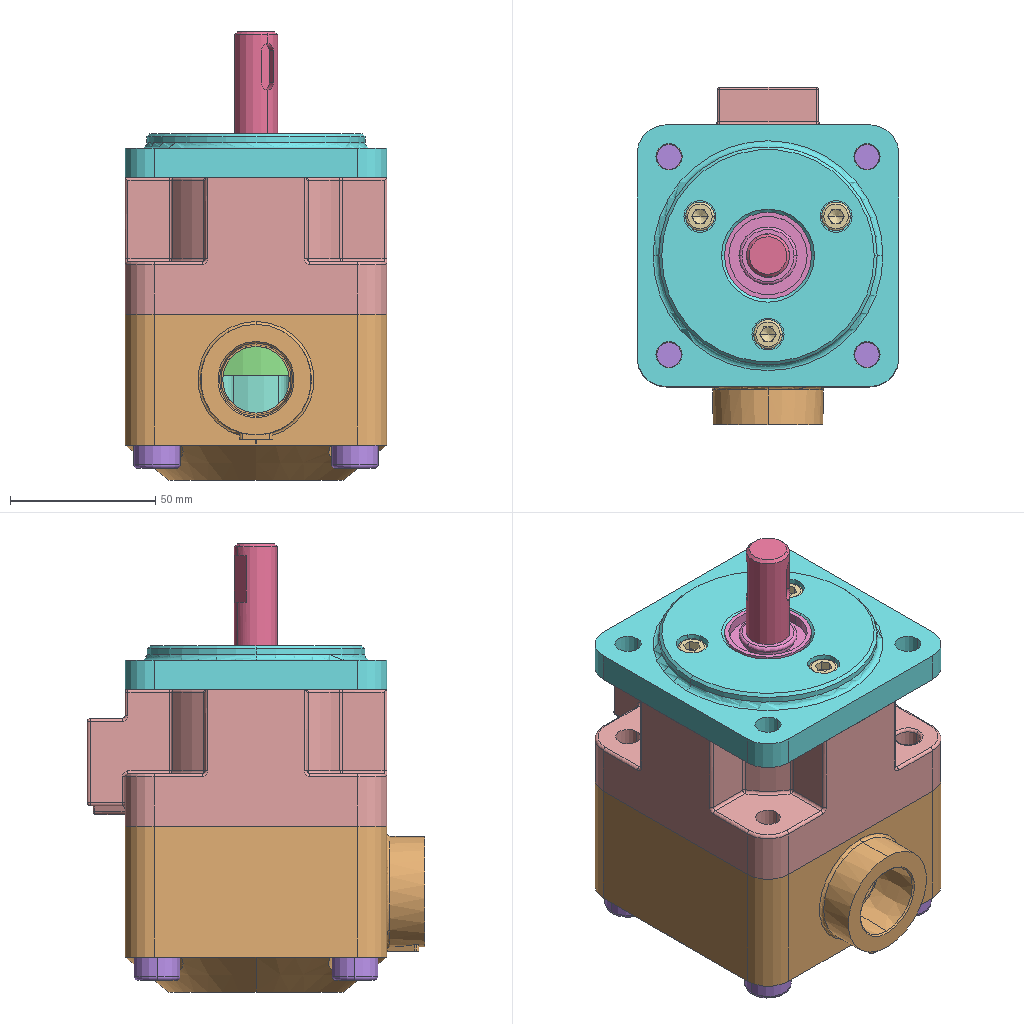Assembly | SolidWorks | 24 different items | 38 placed | box 90 x 116 x 154 mm
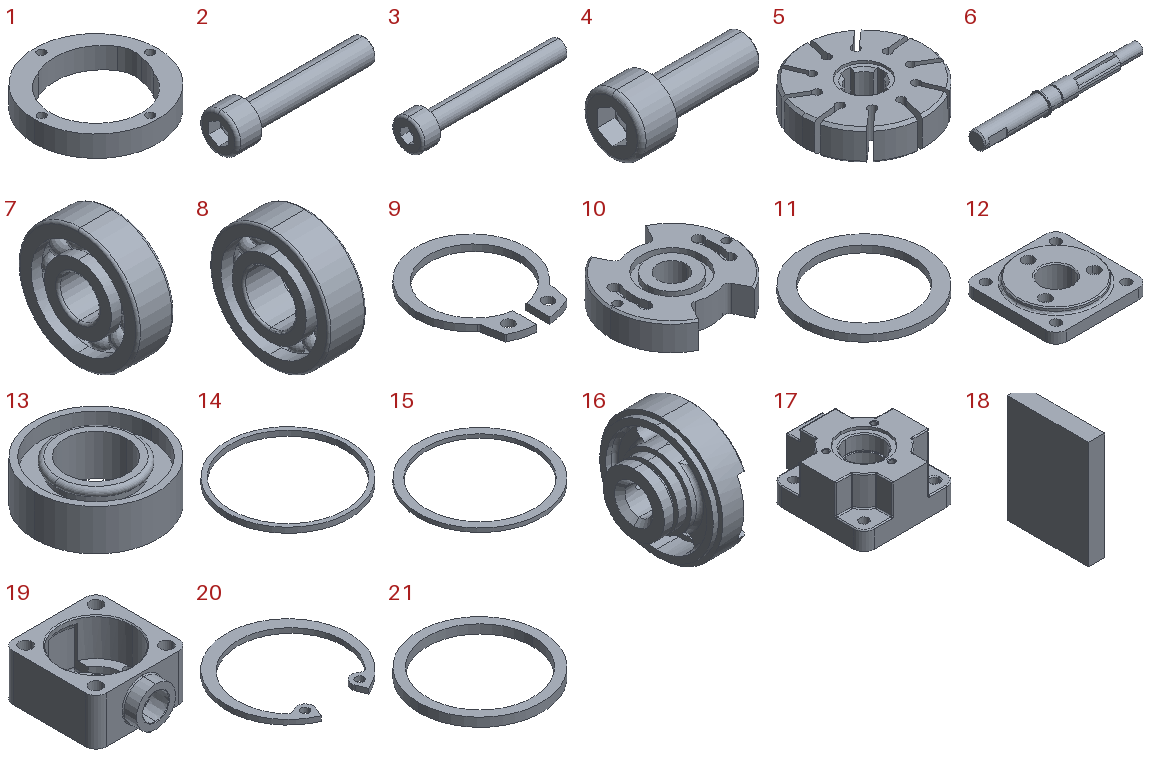Parts list (item | name | quantity | size | volume | features):
1 | - | x1 | 70 x 70 x 12 mm | 19285 mm3 | features Extrusion 1, ICE 1
2 | - | x4 | 60 x 16 x 16 mm | 5603 mm3 | features Fillet 2, RevCut 2, Boss 1, Chamfer 1, Cut 1, Extrusion 1, LPattern 1
3 | - | x1 | 34 x 7 x 7 mm | 511.915 mm3 | features Fillet 2, RevCut 2, Boss 1, Chamfer 1, Cut 1, Extrusion 1, LPattern 1
4 | - | x3 | 22 x 10 x 10 mm | 844.992 mm3 | features Fillet 2, RevCut 2, Boss 1, Chamfer 1, Cut 1, Extrusion 1, LPattern 1
5 | - | x1 | 48 x 48 x 12 mm | 17049 mm3 | features ICE 5, Chamfer 2, CirPattern 1, Extrusion 1
6 | - | x1 | 142 x 18 x 18 mm | 20860 mm3 | features Chamfer 4, ICE 3, Revolution 1
7 | - | x1 | 9 x 30 x 30 mm | 4205 mm3 | features Revolution 3, CirPattern 1, Fillet 1
8 | - | x1 | 11 x 35 x 35 mm | 6320 mm3 | features Revolution 3, CirPattern 1, Fillet 1
9 | - | x1 | 16.8 x 19.352 x 1 mm | 87.473 mm3 | features Fillet 2, Extrusion 1
10 | - | x1 | 70 x 62.37 x 15 mm | 42070 mm3 | features ICE 5, MirrorPattern 2, Chamfer 1, Extrusion 1, Fillet 1
11 | - | x1 | 45 x 45 x 2.5 mm | 1571 mm3 | features Extrusion 1
12 | - | x1 | 90 x 90 x 22 mm | 87928 mm3 | features ICE 6, Fillet 2, Chamfer 1, CirPattern 1, Extrusion 1
13 | - | x1 | 30 x 30 x 10 mm | 3261 mm3 | features MirrorPattern 1, Revolution 1
14 | - | x1 | 70 x 70 x 3 mm | 1590 mm3 | features Extrusion 1
15 | - | x1 | 80 x 80 x 2.5 mm | 2945 mm3 | features Extrusion 1
16 | - | x1 | 33 x 70 x 70 mm | 62726 mm3 | features ICE 5, MirrorPattern 3, Chamfer 2, Fillet 2, 3DProfileFeature 1, HoleWzd 1, Revolution 1
17 | - | x1 | 90 x 103 x 47 mm | 196291 mm3 | features 3DProfileFeature 3, Fillet 3, HoleWzd 3, ICE 3, Chamfer 1, Extrusion 1, RevCut 1
18 | - | x10 | 1.8 x 9 x 12 mm | 184.26 mm3 | features Extrusion 1
19 | - | x1 | 90 x 103 x 57 mm | 228367 mm3 | features ICE 13, Fillet 3, 3DProfileFeature 1, Chamfer 1, CirPattern 1, Extrusion 1, HoleWzd 1, Revolution 1
20 | - | x1 | 37.8 x 36.361 x 1.5 mm | 438.212 mm3 | features Extrusion 1
21 | - | x1 | 35 x 35 x 2.5 mm | 638.136 mm3 | features Extrusion 1
22 | O-Ring 80 | x1 | - | - | -
23 | deep groove ball bearings gb | x1 | - | - | -
24 | hexagon socket head cap screws gb | x1 | - | - | -
Mates (type | each side: item.copy, entity, surface, feature):
Coincident | 5.1 face plane Cut-Extrude 5 | 18.1 face plane Boss-Extrude 1
Coincident | 5.1 face plane Boss-Extrude 1 | 18.1 face plane Boss-Extrude 1
Coincident | 5.1 face plane CirPattern 1 | 18.2 face plane Boss-Extrude 1
Coincident | 5.1 face plane Boss-Extrude 1 | 18.2 face plane Boss-Extrude 1
Coincident | 5.1 face plane CirPattern 1 | 18.3 face plane Boss-Extrude 1
Coincident | 5.1 face plane Boss-Extrude 1 | 18.3 face plane Boss-Extrude 1
Coincident | 5.1 face plane CirPattern 1 | 18.4 face plane Boss-Extrude 1
Coincident | 5.1 face plane Boss-Extrude 1 | 18.4 face plane Boss-Extrude 1
Tangent | 5.1 face cylinder Boss-Extrude 1 | 18.3 face plane Boss-Extrude 1
Tangent | 5.1 face cylinder Boss-Extrude 1 | 18.1 face plane Boss-Extrude 1
Tangent | 5.1 face cylinder Boss-Extrude 1 | 18.2 face plane Boss-Extrude 1
Tangent | 5.1 face cylinder Boss-Extrude 1 | 18.4 face plane Boss-Extrude 1
Coincident | 5.1 face plane CirPattern 1 | 18.5 face plane Boss-Extrude 1
Coincident | 5.1 face plane Boss-Extrude 1 | 18.5 face plane Boss-Extrude 1
Tangent | 5.1 face cylinder Boss-Extrude 1 | 18.5 face plane Boss-Extrude 1
Coincident | 5.1 face plane CirPattern 1 | 18.6 face plane Boss-Extrude 1
Coincident | 5.1 face plane Boss-Extrude 1 | 18.6 face plane Boss-Extrude 1
Coincident | 5.1 face plane CirPattern 1 | 18.7 face plane Boss-Extrude 1
Coincident | 5.1 face plane Boss-Extrude 1 | 18.7 face plane Boss-Extrude 1
Coincident | 5.1 face plane CirPattern 1 | 18.8 face plane Boss-Extrude 1
Coincident | 5.1 face plane Boss-Extrude 1 | 18.8 face plane Boss-Extrude 1
Tangent | 5.1 face cylinder Boss-Extrude 1 | 18.6 face plane Boss-Extrude 1
Tangent | 5.1 face cylinder Boss-Extrude 1 | 18.7 face plane Boss-Extrude 1
Tangent | 5.1 face cylinder Boss-Extrude 1 | 18.8 face plane Boss-Extrude 1
Coincident | 5.1 face plane CirPattern 1 | 18.9 face plane Boss-Extrude 1
Coincident | 5.1 face plane Boss-Extrude 1 | 18.9 face plane Boss-Extrude 1
Coincident | 5.1 face plane CirPattern 1 | 18.10 face plane Boss-Extrude 1
Coincident | 5.1 face plane Boss-Extrude 1 | 18.10 face plane Boss-Extrude 1
Tangent | 5.1 face cylinder Boss-Extrude 1 | 18.10 face plane Boss-Extrude 1
Tangent | 5.1 face cylinder Boss-Extrude 1 | 18.9 face plane Boss-Extrude 1
Concentric | 10.1 face cylinder Cut-Extrude 4 | 19.1 face cone Chamfer 1
Concentric | 10.1 face cylinder Cut-Extrude 5 | 19.1 face cylinder Cut-Extrude 6
Coincident | 10.1 face plane Boss-Extrude 1 | 1.1 face plane Boss-Extrude 1
Concentric | 19.1 face cylinder Cut-Extrude 1 | 1.1 face cylinder Boss-Extrude 1
Concentric | 5.1 face cylinder Cut-Extrude 1 | 6.1 face cylinder Revolve 1
Concentric | 10.1 face cylinder Cut-Extrude 4 | 6.1 face cylinder Revolve 1
Coincident | 5.1 face plane Cut-Extrude 4 | 6.1 face plane Cut-Extrude 1
Coincident | 5.1 face plane Boss-Extrude 1 | 1.1 face plane Boss-Extrude 1
Concentric | 16.1 face cylinder Revolve 1 | 6.1 face cylinder Revolve 1
Concentric | 16.1 face cylinder M4 Tapped Hole 1 | 10.1 face cylinder Cut-Extrude 5
Coincident | 16.1 face plane Revolve 1 | 1.1 face plane Boss-Extrude 1
Concentric | 17.1 face cylinder Cut-Revolve 1 | 15.1 face cylinder Boss-Extrude 1
Coincident | 17.1 face plane Cut-Revolve 1 | 15.1 face plane Boss-Extrude 1
Concentric | 16.1 face cylinder Revolve 1 | 14.1 face cylinder Boss-Extrude 1
Coincident | 16.1 face plane Revolve 1 | 14.1 face plane Boss-Extrude 1
Concentric | 6.1 face cylinder Revolve 1 | 21.1 edge
Coincident | 16.1 face plane Revolve 1 | 21.1 face plane Boss-Extrude 1
Concentric | 17.1 face cylinder Cut-Revolve 1 | 20.1 face cylinder Body
Coincident | 17.1 face plane Cut-Revolve 1 | 20.1 face plane Body
Concentric | 17.1 face cylinder Cut-Revolve 1 | 8.1 face cylinder Revolve3
Coincident | 20.1 face plane Body | 8.1 face plane Revolve3
Concentric | 6.1 face cylinder Revolve 1 | 9.1 face cylinder Body
Concentric | 17.1 face cylinder Cut-Revolve 1 | 6.1 face cylinder Revolve 1
Concentric | 17.1 face cylinder M10 Tapped Hole 1 | 19.1 face cylinder CirPattern 2
Coincident | 6.1 face plane Revolve 1 | 9.1 face plane Body
Coincident | 17.1 face plane Boss-Extrude 1 | 19.1 face plane Boss-Extrude 1
Concentric | 6.1 face cylinder Revolve 1 | 12.1 face cylinder Boss-Extrude 3
Concentric | 17.1 face cylinder M6 Tapped Hole 1 | 12.1 face cylinder Cut-Extrude 3
Coincident | 17.1 face plane Boss-Extrude 2 | 12.1 face plane Boss-Extrude 1
Concentric | 13.1 face cylinder Revolve 2 | 12.1 face cylinder Cut-Extrude 2
Coincident | 13.1 edge | 12.1 face plane Boss-Extrude 2
Concentric | 12.1 face cylinder CirPattern 1 | 4.1 face cylinder BaseBody
Concentric | 12.1 face cylinder CirPattern 1 | 4.2 face cylinder BaseHead
Concentric | 12.1 face cylinder Cut-Extrude 3 | 4.3 face cylinder BaseHead
Coincident | 12.1 face plane CirPattern 1 | 4.1 edge
Coincident | 12.1 face plane CirPattern 1 | 4.2 face plane BaseHead
Coincident | 12.1 face plane Cut-Extrude 3 | 4.3 face plane BaseHead
Concentric | 19.1 face cylinder CirPattern 2 | 2.1 face cylinder BaseBody
Concentric | 19.1 face cylinder Cut-Extrude 8 | 2.2 face cylinder BaseBody
Concentric | 19.1 face cylinder CirPattern 2 | 2.3 face cylinder BaseBody
Concentric | 19.1 face cylinder CirPattern 2 | 2.4 face cylinder BaseBody
Coincident | 19.1 face plane CirPattern 2 | 2.4 face plane BaseHead
Coincident | 19.1 face plane CirPattern 2 | 2.3 face plane BaseHead
Coincident | 19.1 face plane CirPattern 2 | 2.1 face plane BaseHead
Coincident | 19.1 edge | 2.2 face plane BaseHead